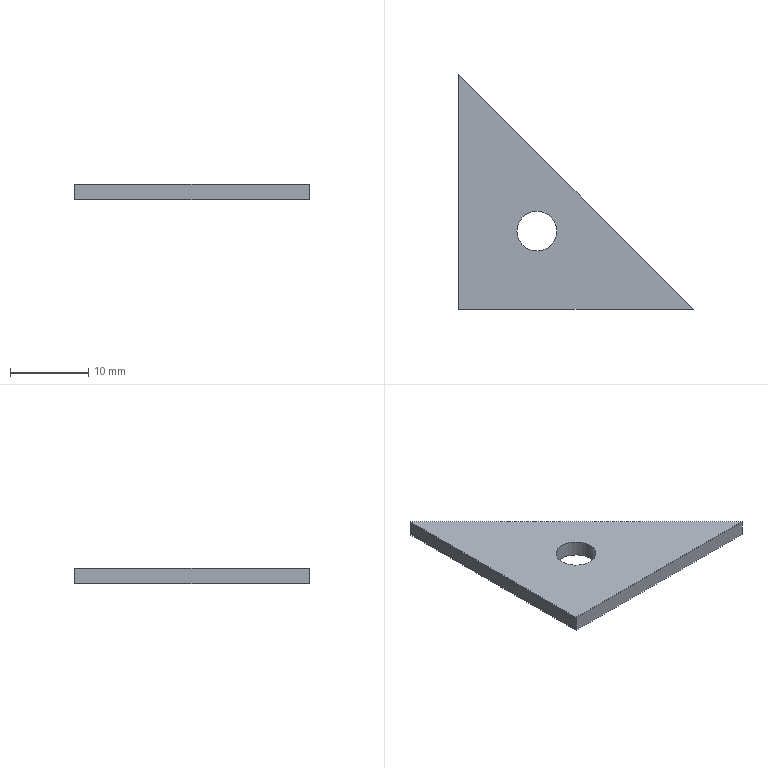Part | SolidWorks | features FlatPattern 1, SMBaseFlange 1, SheetMetal 1 | 1 solid | 7 faces | box 30 x 30 x 2 mm | volume 859.144 mm3 | plane 5 | cylinder 2 | commonest cylinder face diameters 5.1 x2
STEP:
#1=CARTESIAN_POINT('',(7.45,10.,-2.));
#2=VERTEX_POINT('',#1);
#3=CARTESIAN_POINT('',(12.55,10.,-2.));
#4=VERTEX_POINT('',#3);
#5=CARTESIAN_POINT('',(10.,10.,-2.));
#6=DIRECTION('',(0.,0.,1.));
#7=DIRECTION('',(1.,0.,0.));
#8=AXIS2_PLACEMENT_3D('',#5,#6,#7);
#9=CIRCLE('',#8,2.55);
#10=EDGE_CURVE('',#2,#4,#9,.T.);
#11=ORIENTED_EDGE('',*,*,#10,.F.);
#12=CARTESIAN_POINT('',(7.45,10.,0.));
#13=VERTEX_POINT('',#12);
#14=CARTESIAN_POINT('',(7.45,10.,-2.));
#15=DIRECTION('',(0.,0.,1.));
#16=VECTOR('',#15,1000.);
#17=LINE('',#14,#16);
#18=EDGE_CURVE('',#2,#13,#17,.T.);
#19=ORIENTED_EDGE('',*,*,#18,.T.);
#20=CARTESIAN_POINT('',(12.55,10.,0.));
#21=VERTEX_POINT('',#20);
#22=CARTESIAN_POINT('',(10.,10.,0.));
#23=DIRECTION('',(0.,0.,1.));
#24=DIRECTION('',(1.,0.,0.));
#25=AXIS2_PLACEMENT_3D('',#22,#23,#24);
#26=CIRCLE('',#25,2.55);
#27=EDGE_CURVE('',#13,#21,#26,.T.);
#28=ORIENTED_EDGE('',*,*,#27,.T.);
#29=CARTESIAN_POINT('',(12.55,10.,-2.));
#30=DIRECTION('',(0.,0.,1.));
#31=VECTOR('',#30,1000.);
#32=LINE('',#29,#31);
#33=EDGE_CURVE('',#4,#21,#32,.T.);
#34=ORIENTED_EDGE('',*,*,#33,.F.);
#35=EDGE_LOOP('',(#11,#19,#28,#34));
#36=FACE_OUTER_BOUND('',#35,.T.);
#37=CARTESIAN_POINT('',(10.,10.,-2.));
#38=DIRECTION('',(0.,0.,1.));
#39=DIRECTION('',(1.,0.,0.));
#40=AXIS2_PLACEMENT_3D('',#37,#38,#39);
#41=CYLINDRICAL_SURFACE('',#40,2.55);
#42=ADVANCED_FACE('',(#36),#41,.F.);
#43=CARTESIAN_POINT('',(30.,0.,0.));
#44=VERTEX_POINT('',#43);
#45=CARTESIAN_POINT('',(0.,30.,0.));
#46=VERTEX_POINT('',#45);
#47=CARTESIAN_POINT('',(30.,0.,0.));
#48=DIRECTION('',(-0.7071,0.7071,0.));
#49=VECTOR('',#48,1000.);
#50=LINE('',#47,#49);
#51=EDGE_CURVE('',#44,#46,#50,.T.);
#52=ORIENTED_EDGE('',*,*,#51,.F.);
#53=CARTESIAN_POINT('',(30.,0.,-2.));
#54=VERTEX_POINT('',#53);
#55=CARTESIAN_POINT('',(30.,0.,-2.));
#56=DIRECTION('',(0.,0.,1.));
#57=VECTOR('',#56,1000.);
#58=LINE('',#55,#57);
#59=EDGE_CURVE('',#54,#44,#58,.T.);
#60=ORIENTED_EDGE('',*,*,#59,.F.);
#61=CARTESIAN_POINT('',(0.,30.,-2.));
#62=VERTEX_POINT('',#61);
#63=CARTESIAN_POINT('',(30.,0.,-2.));
#64=DIRECTION('',(-0.7071,0.7071,0.));
#65=VECTOR('',#64,1000.);
#66=LINE('',#63,#65);
#67=EDGE_CURVE('',#54,#62,#66,.T.);
#68=ORIENTED_EDGE('',*,*,#67,.T.);
#69=CARTESIAN_POINT('',(0.,30.,-2.));
#70=DIRECTION('',(0.,0.,1.));
#71=VECTOR('',#70,1000.);
#72=LINE('',#69,#71);
#73=EDGE_CURVE('',#62,#46,#72,.T.);
#74=ORIENTED_EDGE('',*,*,#73,.T.);
#75=EDGE_LOOP('',(#52,#60,#68,#74));
#76=FACE_OUTER_BOUND('',#75,.T.);
#77=CARTESIAN_POINT('',(30.,0.,-2.));
#78=DIRECTION('',(0.7071,0.7071,0.));
#79=DIRECTION('',(-0.7071,0.7071,0.));
#80=AXIS2_PLACEMENT_3D('',#77,#78,#79);
#81=PLANE('',#80);
#82=ADVANCED_FACE('',(#76),#81,.T.);
#83=CARTESIAN_POINT('',(0.,0.,0.));
#84=VERTEX_POINT('',#83);
#85=CARTESIAN_POINT('',(0.,0.,0.));
#86=DIRECTION('',(1.,0.,0.));
#87=VECTOR('',#86,1000.);
#88=LINE('',#85,#87);
#89=EDGE_CURVE('',#84,#44,#88,.T.);
#90=ORIENTED_EDGE('',*,*,#89,.F.);
#91=CARTESIAN_POINT('',(0.,0.,-2.));
#92=VERTEX_POINT('',#91);
#93=CARTESIAN_POINT('',(0.,0.,-2.));
#94=DIRECTION('',(0.,0.,1.));
#95=VECTOR('',#94,1000.);
#96=LINE('',#93,#95);
#97=EDGE_CURVE('',#92,#84,#96,.T.);
#98=ORIENTED_EDGE('',*,*,#97,.F.);
#99=CARTESIAN_POINT('',(0.,0.,-2.));
#100=DIRECTION('',(1.,0.,0.));
#101=VECTOR('',#100,1000.);
#102=LINE('',#99,#101);
#103=EDGE_CURVE('',#92,#54,#102,.T.);
#104=ORIENTED_EDGE('',*,*,#103,.T.);
#105=ORIENTED_EDGE('',*,*,#59,.T.);
#106=EDGE_LOOP('',(#90,#98,#104,#105));
#107=FACE_OUTER_BOUND('',#106,.T.);
#108=CARTESIAN_POINT('',(0.,0.,-2.));
#109=DIRECTION('',(0.,-1.,0.));
#110=DIRECTION('',(0.,0.,-1.));
#111=AXIS2_PLACEMENT_3D('',#108,#109,#110);
#112=PLANE('',#111);
#113=ADVANCED_FACE('',(#107),#112,.T.);
#114=CARTESIAN_POINT('',(0.,30.,0.));
#115=DIRECTION('',(0.,-1.,0.));
#116=VECTOR('',#115,1000.);
#117=LINE('',#114,#116);
#118=EDGE_CURVE('',#46,#84,#117,.T.);
#119=ORIENTED_EDGE('',*,*,#118,.F.);
#120=ORIENTED_EDGE('',*,*,#73,.F.);
#121=CARTESIAN_POINT('',(0.,30.,-2.));
#122=DIRECTION('',(0.,-1.,0.));
#123=VECTOR('',#122,1000.);
#124=LINE('',#121,#123);
#125=EDGE_CURVE('',#62,#92,#124,.T.);
#126=ORIENTED_EDGE('',*,*,#125,.T.);
#127=ORIENTED_EDGE('',*,*,#97,.T.);
#128=EDGE_LOOP('',(#119,#120,#126,#127));
#129=FACE_OUTER_BOUND('',#128,.T.);
#130=CARTESIAN_POINT('',(0.,30.,-2.));
#131=DIRECTION('',(-1.,0.,0.));
#132=DIRECTION('',(0.,-1.,0.));
#133=AXIS2_PLACEMENT_3D('',#130,#131,#132);
#134=PLANE('',#133);
#135=ADVANCED_FACE('',(#129),#134,.T.);
#136=CARTESIAN_POINT('',(10.,10.,-2.));
#137=DIRECTION('',(0.,0.,1.));
#138=DIRECTION('',(1.,0.,0.));
#139=AXIS2_PLACEMENT_3D('',#136,#137,#138);
#140=CIRCLE('',#139,2.55);
#141=EDGE_CURVE('',#4,#2,#140,.T.);
#142=ORIENTED_EDGE('',*,*,#141,.T.);
#143=ORIENTED_EDGE('',*,*,#10,.T.);
#144=EDGE_LOOP('',(#142,#143));
#145=FACE_BOUND('',#144,.T.);
#146=ORIENTED_EDGE('',*,*,#67,.F.);
#147=ORIENTED_EDGE('',*,*,#103,.F.);
#148=ORIENTED_EDGE('',*,*,#125,.F.);
#149=EDGE_LOOP('',(#146,#147,#148));
#150=FACE_OUTER_BOUND('',#149,.T.);
#151=CARTESIAN_POINT('',(0.,0.,-2.));
#152=DIRECTION('',(0.,0.,1.));
#153=DIRECTION('',(1.,0.,0.));
#154=AXIS2_PLACEMENT_3D('',#151,#152,#153);
#155=PLANE('',#154);
#156=ADVANCED_FACE('',(#145,#150),#155,.F.);
#157=CARTESIAN_POINT('',(10.,10.,0.));
#158=DIRECTION('',(0.,0.,1.));
#159=DIRECTION('',(1.,0.,0.));
#160=AXIS2_PLACEMENT_3D('',#157,#158,#159);
#161=CIRCLE('',#160,2.55);
#162=EDGE_CURVE('',#21,#13,#161,.T.);
#163=ORIENTED_EDGE('',*,*,#162,.F.);
#164=ORIENTED_EDGE('',*,*,#27,.F.);
#165=EDGE_LOOP('',(#163,#164));
#166=FACE_BOUND('',#165,.T.);
#167=ORIENTED_EDGE('',*,*,#51,.T.);
#168=ORIENTED_EDGE('',*,*,#118,.T.);
#169=ORIENTED_EDGE('',*,*,#89,.T.);
#170=EDGE_LOOP('',(#167,#168,#169));
#171=FACE_OUTER_BOUND('',#170,.T.);
#172=CARTESIAN_POINT('',(0.,0.,0.));
#173=DIRECTION('',(0.,0.,1.));
#174=DIRECTION('',(1.,0.,0.));
#175=AXIS2_PLACEMENT_3D('',#172,#173,#174);
#176=PLANE('',#175);
#177=ADVANCED_FACE('',(#166,#171),#176,.T.);
#178=ORIENTED_EDGE('',*,*,#18,.F.);
#179=ORIENTED_EDGE('',*,*,#141,.F.);
#180=ORIENTED_EDGE('',*,*,#33,.T.);
#181=ORIENTED_EDGE('',*,*,#162,.T.);
#182=EDGE_LOOP('',(#178,#179,#180,#181));
#183=FACE_OUTER_BOUND('',#182,.T.);
#184=CARTESIAN_POINT('',(10.,10.,-2.));
#185=DIRECTION('',(0.,0.,1.));
#186=DIRECTION('',(1.,0.,0.));
#187=AXIS2_PLACEMENT_3D('',#184,#185,#186);
#188=CYLINDRICAL_SURFACE('',#187,2.55);
#189=ADVANCED_FACE('',(#183),#188,.F.);
#190=CLOSED_SHELL('',(#42,#82,#113,#135,#156,#177,#189));
#191=MANIFOLD_SOLID_BREP('',#190);
#192=CARTESIAN_POINT('',(0.,0.,0.));
#193=DIRECTION('',(0.,0.,1.));
#194=DIRECTION('',(1.,0.,0.));
#195=AXIS2_PLACEMENT_3D('',#192,#193,#194);
#196=(LENGTH_UNIT()NAMED_UNIT(*)SI_UNIT(.MILLI.,.METRE.));
#197=UNCERTAINTY_MEASURE_WITH_UNIT(LENGTH_MEASURE(0.00001),#196,'','');
#198=(NAMED_UNIT(*)PLANE_ANGLE_UNIT()SI_UNIT($,.RADIAN.));
#199=(NAMED_UNIT(*)SI_UNIT($,.STERADIAN.)SOLID_ANGLE_UNIT());
#200=(GEOMETRIC_REPRESENTATION_CONTEXT(3)GLOBAL_UNCERTAINTY_ASSIGNED_CONTEXT((#197))GLOBAL_UNIT_ASSIGNED_CONTEXT((#196,#198,#199))REPRESENTATION_CONTEXT('',''));
#201=ADVANCED_BREP_SHAPE_REPRESENTATION('',(#191,#195),#200);